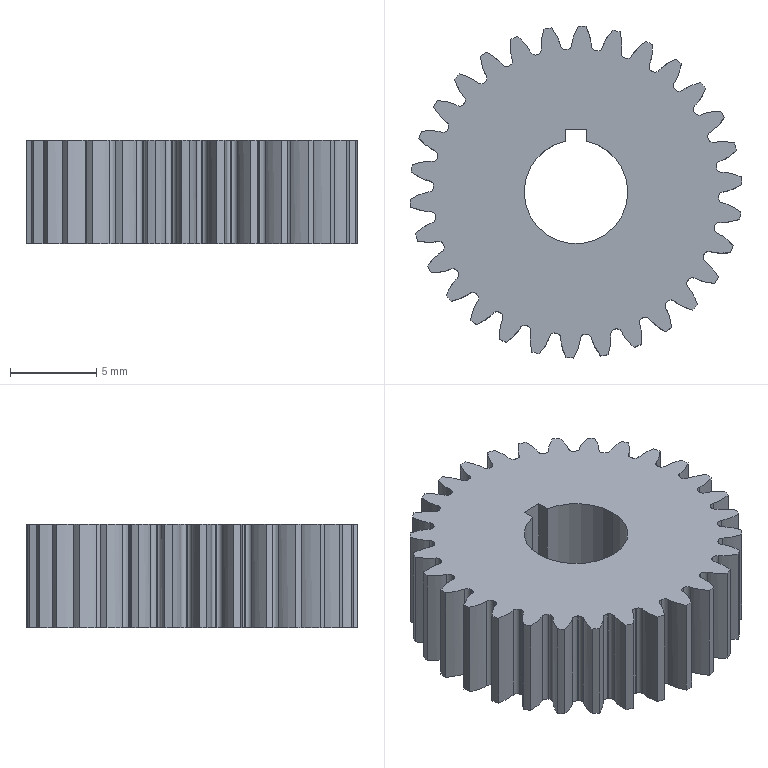Part | SolidWorks | features BaseBody 1, Scale 1 | 1 solid | 201 faces | box 19.181 x 19.198 x 6 mm | volume 1338 mm3 | cylinder 136 | spline 60 | plane 5 | commonest cylinder face diameters 0.6 x73 16.5 x30 19.2 x30 6 x3